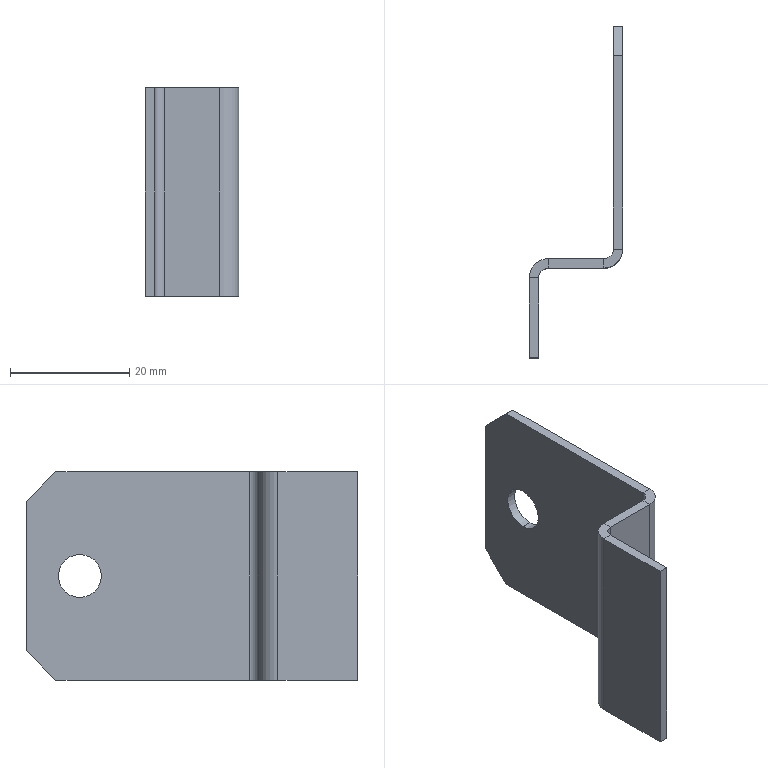Part | SolidWorks | features Chamfer 2, FlatPattern 1, ICE 1, SMBaseFlange 1, SheetMetal 1 | 1 solid | 26 faces | box 15.7 x 55.6 x 35 mm | volume 3683 mm3 | plane 20 | cylinder 6 | commonest cylinder face diameters 3.2 x2 6.4 x2 7.2 x2
STEP:
#1=CARTESIAN_POINT('',(-1.6,47.021,-13.9));
#2=VERTEX_POINT('',#1);
#3=CARTESIAN_POINT('',(-1.6,47.021,-21.1));
#4=VERTEX_POINT('',#3);
#5=CARTESIAN_POINT('',(-1.6,47.021,-17.5));
#6=DIRECTION('',(1.,0.,0.));
#7=DIRECTION('',(0.,0.,-1.));
#8=AXIS2_PLACEMENT_3D('',#5,#6,#7);
#9=CIRCLE('',#8,3.6);
#10=EDGE_CURVE('',#2,#4,#9,.T.);
#11=ORIENTED_EDGE('',*,*,#10,.F.);
#12=CARTESIAN_POINT('',(0.,47.021,-13.9));
#13=VERTEX_POINT('',#12);
#14=CARTESIAN_POINT('',(-1.6,47.021,-13.9));
#15=DIRECTION('',(1.,0.,0.));
#16=VECTOR('',#15,1000.);
#17=LINE('',#14,#16);
#18=EDGE_CURVE('',#2,#13,#17,.T.);
#19=ORIENTED_EDGE('',*,*,#18,.T.);
#20=CARTESIAN_POINT('',(0.,47.021,-21.1));
#21=VERTEX_POINT('',#20);
#22=CARTESIAN_POINT('',(0.,47.021,-17.5));
#23=DIRECTION('',(1.,0.,0.));
#24=DIRECTION('',(0.,0.,-1.));
#25=AXIS2_PLACEMENT_3D('',#22,#23,#24);
#26=CIRCLE('',#25,3.6);
#27=EDGE_CURVE('',#13,#21,#26,.T.);
#28=ORIENTED_EDGE('',*,*,#27,.T.);
#29=CARTESIAN_POINT('',(-1.6,47.021,-21.1));
#30=DIRECTION('',(1.,0.,0.));
#31=VECTOR('',#30,1000.);
#32=LINE('',#29,#31);
#33=EDGE_CURVE('',#4,#21,#32,.T.);
#34=ORIENTED_EDGE('',*,*,#33,.F.);
#35=EDGE_LOOP('',(#11,#19,#28,#34));
#36=FACE_OUTER_BOUND('',#35,.T.);
#37=CARTESIAN_POINT('',(-1.6,47.021,-17.5));
#38=DIRECTION('',(1.,0.,0.));
#39=DIRECTION('',(0.,0.,-1.));
#40=AXIS2_PLACEMENT_3D('',#37,#38,#39);
#41=CYLINDRICAL_SURFACE('',#40,3.6);
#42=ADVANCED_FACE('',(#36),#41,.F.);
#43=CARTESIAN_POINT('',(0.,18.621,-35.));
#44=VERTEX_POINT('',#43);
#45=CARTESIAN_POINT('',(-1.6,18.621,-35.));
#46=VERTEX_POINT('',#45);
#47=CARTESIAN_POINT('',(0.,18.621,-35.));
#48=DIRECTION('',(-1.,0.,0.));
#49=VECTOR('',#48,1000.);
#50=LINE('',#47,#49);
#51=EDGE_CURVE('',#44,#46,#50,.T.);
#52=ORIENTED_EDGE('',*,*,#51,.F.);
#53=CARTESIAN_POINT('',(-3.2,15.421,-35.));
#54=VERTEX_POINT('',#53);
#55=CARTESIAN_POINT('',(-3.2,18.621,-35.));
#56=DIRECTION('',(0.,0.,-1.));
#57=DIRECTION('',(1.,0.,0.));
#58=AXIS2_PLACEMENT_3D('',#55,#56,#57);
#59=CIRCLE('',#58,3.2);
#60=EDGE_CURVE('',#44,#54,#59,.T.);
#61=ORIENTED_EDGE('',*,*,#60,.T.);
#62=CARTESIAN_POINT('',(-3.2,17.021,-35.));
#63=VERTEX_POINT('',#62);
#64=CARTESIAN_POINT('',(-3.2,17.021,-35.));
#65=DIRECTION('',(0.,-1.,0.));
#66=VECTOR('',#65,1000.);
#67=LINE('',#64,#66);
#68=EDGE_CURVE('',#63,#54,#67,.T.);
#69=ORIENTED_EDGE('',*,*,#68,.F.);
#70=CARTESIAN_POINT('',(-3.2,18.621,-35.));
#71=DIRECTION('',(0.,0.,-1.));
#72=DIRECTION('',(1.,0.,0.));
#73=AXIS2_PLACEMENT_3D('',#70,#71,#72);
#74=CIRCLE('',#73,1.6);
#75=EDGE_CURVE('',#46,#63,#74,.T.);
#76=ORIENTED_EDGE('',*,*,#75,.F.);
#77=EDGE_LOOP('',(#52,#61,#69,#76));
#78=FACE_OUTER_BOUND('',#77,.T.);
#79=CARTESIAN_POINT('',(0.,18.621,-35.));
#80=DIRECTION('',(0.,0.,-1.));
#81=DIRECTION('',(-1.,0.,0.));
#82=AXIS2_PLACEMENT_3D('',#79,#80,#81);
#83=PLANE('',#82);
#84=ADVANCED_FACE('',(#78),#83,.T.);
#85=CARTESIAN_POINT('',(-1.6,51.021,-35.));
#86=VERTEX_POINT('',#85);
#87=CARTESIAN_POINT('',(-1.6,56.021,-35.));
#88=DIRECTION('',(0.,-1.,0.));
#89=VECTOR('',#88,1000.);
#90=LINE('',#87,#89);
#91=EDGE_CURVE('',#86,#46,#90,.T.);
#92=ORIENTED_EDGE('',*,*,#91,.F.);
#93=CARTESIAN_POINT('',(0.,51.021,-35.));
#94=VERTEX_POINT('',#93);
#95=CARTESIAN_POINT('',(0.,51.021,-35.));
#96=DIRECTION('',(1.,0.,0.));
#97=VECTOR('',#96,1000.);
#98=LINE('',#95,#97);
#99=EDGE_CURVE('',#86,#94,#98,.T.);
#100=ORIENTED_EDGE('',*,*,#99,.T.);
#101=CARTESIAN_POINT('',(0.,56.021,-35.));
#102=DIRECTION('',(0.,-1.,0.));
#103=VECTOR('',#102,1000.);
#104=LINE('',#101,#103);
#105=EDGE_CURVE('',#94,#44,#104,.T.);
#106=ORIENTED_EDGE('',*,*,#105,.T.);
#107=ORIENTED_EDGE('',*,*,#51,.T.);
#108=EDGE_LOOP('',(#92,#100,#106,#107));
#109=FACE_OUTER_BOUND('',#108,.T.);
#110=CARTESIAN_POINT('',(-3.2,17.021,-35.));
#111=DIRECTION('',(0.,0.,-1.));
#112=DIRECTION('',(-1.,0.,0.));
#113=AXIS2_PLACEMENT_3D('',#110,#111,#112);
#114=PLANE('',#113);
#115=ADVANCED_FACE('',(#109),#114,.T.);
#116=CARTESIAN_POINT('',(-3.2,15.421,0.));
#117=VERTEX_POINT('',#116);
#118=CARTESIAN_POINT('',(-3.2,17.021,0.));
#119=VERTEX_POINT('',#118);
#120=CARTESIAN_POINT('',(-3.2,15.421,0.));
#121=DIRECTION('',(0.,1.,0.));
#122=VECTOR('',#121,1000.);
#123=LINE('',#120,#122);
#124=EDGE_CURVE('',#117,#119,#123,.T.);
#125=ORIENTED_EDGE('',*,*,#124,.F.);
#126=CARTESIAN_POINT('',(0.,18.621,0.));
#127=VERTEX_POINT('',#126);
#128=CARTESIAN_POINT('',(-3.2,18.621,0.));
#129=DIRECTION('',(0.,0.,-1.));
#130=DIRECTION('',(1.,0.,0.));
#131=AXIS2_PLACEMENT_3D('',#128,#129,#130);
#132=CIRCLE('',#131,3.2);
#133=EDGE_CURVE('',#127,#117,#132,.T.);
#134=ORIENTED_EDGE('',*,*,#133,.F.);
#135=CARTESIAN_POINT('',(-1.6,18.621,0.));
#136=VERTEX_POINT('',#135);
#137=CARTESIAN_POINT('',(-1.6,18.621,0.));
#138=DIRECTION('',(1.,0.,0.));
#139=VECTOR('',#138,1000.);
#140=LINE('',#137,#139);
#141=EDGE_CURVE('',#136,#127,#140,.T.);
#142=ORIENTED_EDGE('',*,*,#141,.F.);
#143=CARTESIAN_POINT('',(-3.2,18.621,0.));
#144=DIRECTION('',(0.,0.,-1.));
#145=DIRECTION('',(1.,0.,0.));
#146=AXIS2_PLACEMENT_3D('',#143,#144,#145);
#147=CIRCLE('',#146,1.6);
#148=EDGE_CURVE('',#136,#119,#147,.T.);
#149=ORIENTED_EDGE('',*,*,#148,.T.);
#150=EDGE_LOOP('',(#125,#134,#142,#149));
#151=FACE_OUTER_BOUND('',#150,.T.);
#152=CARTESIAN_POINT('',(-3.2,15.421,0.));
#153=DIRECTION('',(0.,0.,1.));
#154=DIRECTION('',(1.,0.,0.));
#155=AXIS2_PLACEMENT_3D('',#152,#153,#154);
#156=PLANE('',#155);
#157=ADVANCED_FACE('',(#151),#156,.T.);
#158=CARTESIAN_POINT('',(-12.5,15.421,0.));
#159=VERTEX_POINT('',#158);
#160=CARTESIAN_POINT('',(0.,15.421,0.));
#161=DIRECTION('',(-1.,0.,0.));
#162=VECTOR('',#161,1000.);
#163=LINE('',#160,#162);
#164=EDGE_CURVE('',#117,#159,#163,.T.);
#165=ORIENTED_EDGE('',*,*,#164,.F.);
#166=ORIENTED_EDGE('',*,*,#124,.T.);
#167=CARTESIAN_POINT('',(-12.5,17.021,0.));
#168=VERTEX_POINT('',#167);
#169=CARTESIAN_POINT('',(0.,17.021,0.));
#170=DIRECTION('',(-1.,0.,0.));
#171=VECTOR('',#170,1000.);
#172=LINE('',#169,#171);
#173=EDGE_CURVE('',#119,#168,#172,.T.);
#174=ORIENTED_EDGE('',*,*,#173,.T.);
#175=CARTESIAN_POINT('',(-12.5,17.021,0.));
#176=DIRECTION('',(0.,-1.,0.));
#177=VECTOR('',#176,1000.);
#178=LINE('',#175,#177);
#179=EDGE_CURVE('',#168,#159,#178,.T.);
#180=ORIENTED_EDGE('',*,*,#179,.T.);
#181=EDGE_LOOP('',(#165,#166,#174,#180));
#182=FACE_OUTER_BOUND('',#181,.T.);
#183=CARTESIAN_POINT('',(-1.6,18.621,0.));
#184=DIRECTION('',(0.,0.,1.));
#185=DIRECTION('',(1.,0.,0.));
#186=AXIS2_PLACEMENT_3D('',#183,#184,#185);
#187=PLANE('',#186);
#188=ADVANCED_FACE('',(#182),#187,.T.);
#189=CARTESIAN_POINT('',(-12.5,15.421,-35.));
#190=VERTEX_POINT('',#189);
#191=CARTESIAN_POINT('',(-12.5,17.021,-35.));
#192=VERTEX_POINT('',#191);
#193=CARTESIAN_POINT('',(-12.5,15.421,-35.));
#194=DIRECTION('',(0.,1.,0.));
#195=VECTOR('',#194,1000.);
#196=LINE('',#193,#195);
#197=EDGE_CURVE('',#190,#192,#196,.T.);
#198=ORIENTED_EDGE('',*,*,#197,.F.);
#199=CARTESIAN_POINT('',(-14.1,13.821,-35.));
#200=VERTEX_POINT('',#199);
#201=CARTESIAN_POINT('',(-12.5,13.821,-35.));
#202=DIRECTION('',(0.,0.,1.));
#203=DIRECTION('',(-1.,0.,0.));
#204=AXIS2_PLACEMENT_3D('',#201,#202,#203);
#205=CIRCLE('',#204,1.6);
#206=EDGE_CURVE('',#190,#200,#205,.T.);
#207=ORIENTED_EDGE('',*,*,#206,.T.);
#208=CARTESIAN_POINT('',(-15.7,13.821,-35.));
#209=VERTEX_POINT('',#208);
#210=CARTESIAN_POINT('',(-15.7,13.821,-35.));
#211=DIRECTION('',(1.,0.,0.));
#212=VECTOR('',#211,1000.);
#213=LINE('',#210,#212);
#214=EDGE_CURVE('',#209,#200,#213,.T.);
#215=ORIENTED_EDGE('',*,*,#214,.F.);
#216=CARTESIAN_POINT('',(-12.5,13.821,-35.));
#217=DIRECTION('',(0.,0.,1.));
#218=DIRECTION('',(1.,0.,0.));
#219=AXIS2_PLACEMENT_3D('',#216,#217,#218);
#220=CIRCLE('',#219,3.2);
#221=EDGE_CURVE('',#192,#209,#220,.T.);
#222=ORIENTED_EDGE('',*,*,#221,.F.);
#223=EDGE_LOOP('',(#198,#207,#215,#222));
#224=FACE_OUTER_BOUND('',#223,.T.);
#225=CARTESIAN_POINT('',(-12.5,15.421,-35.));
#226=DIRECTION('',(0.,0.,-1.));
#227=DIRECTION('',(-1.,0.,0.));
#228=AXIS2_PLACEMENT_3D('',#225,#226,#227);
#229=PLANE('',#228);
#230=ADVANCED_FACE('',(#224),#229,.T.);
#231=CARTESIAN_POINT('',(0.,15.421,-35.));
#232=DIRECTION('',(-1.,0.,0.));
#233=VECTOR('',#232,1000.);
#234=LINE('',#231,#233);
#235=EDGE_CURVE('',#54,#190,#234,.T.);
#236=ORIENTED_EDGE('',*,*,#235,.T.);
#237=ORIENTED_EDGE('',*,*,#197,.T.);
#238=CARTESIAN_POINT('',(0.,17.021,-35.));
#239=DIRECTION('',(-1.,0.,0.));
#240=VECTOR('',#239,1000.);
#241=LINE('',#238,#240);
#242=EDGE_CURVE('',#63,#192,#241,.T.);
#243=ORIENTED_EDGE('',*,*,#242,.F.);
#244=ORIENTED_EDGE('',*,*,#68,.T.);
#245=EDGE_LOOP('',(#236,#237,#243,#244));
#246=FACE_OUTER_BOUND('',#245,.T.);
#247=CARTESIAN_POINT('',(-15.7,13.821,-35.));
#248=DIRECTION('',(0.,0.,-1.));
#249=DIRECTION('',(-1.,0.,0.));
#250=AXIS2_PLACEMENT_3D('',#247,#248,#249);
#251=PLANE('',#250);
#252=ADVANCED_FACE('',(#246),#251,.T.);
#253=CARTESIAN_POINT('',(-14.1,13.821,0.));
#254=VERTEX_POINT('',#253);
#255=CARTESIAN_POINT('',(-15.7,13.821,0.));
#256=VERTEX_POINT('',#255);
#257=CARTESIAN_POINT('',(-14.1,13.821,0.));
#258=DIRECTION('',(-1.,0.,0.));
#259=VECTOR('',#258,1000.);
#260=LINE('',#257,#259);
#261=EDGE_CURVE('',#254,#256,#260,.T.);
#262=ORIENTED_EDGE('',*,*,#261,.F.);
#263=CARTESIAN_POINT('',(-12.5,13.821,0.));
#264=DIRECTION('',(0.,0.,1.));
#265=DIRECTION('',(-1.,0.,0.));
#266=AXIS2_PLACEMENT_3D('',#263,#264,#265);
#267=CIRCLE('',#266,1.6);
#268=EDGE_CURVE('',#159,#254,#267,.T.);
#269=ORIENTED_EDGE('',*,*,#268,.F.);
#270=ORIENTED_EDGE('',*,*,#179,.F.);
#271=CARTESIAN_POINT('',(-12.5,13.821,0.));
#272=DIRECTION('',(0.,0.,1.));
#273=DIRECTION('',(1.,0.,0.));
#274=AXIS2_PLACEMENT_3D('',#271,#272,#273);
#275=CIRCLE('',#274,3.2);
#276=EDGE_CURVE('',#168,#256,#275,.T.);
#277=ORIENTED_EDGE('',*,*,#276,.T.);
#278=EDGE_LOOP('',(#262,#269,#270,#277));
#279=FACE_OUTER_BOUND('',#278,.T.);
#280=CARTESIAN_POINT('',(-14.1,13.821,0.));
#281=DIRECTION('',(0.,0.,1.));
#282=DIRECTION('',(1.,0.,0.));
#283=AXIS2_PLACEMENT_3D('',#280,#281,#282);
#284=PLANE('',#283);
#285=ADVANCED_FACE('',(#279),#284,.T.);
#286=CARTESIAN_POINT('',(-14.1,0.4211,0.));
#287=VERTEX_POINT('',#286);
#288=CARTESIAN_POINT('',(-14.1,15.421,0.));
#289=DIRECTION('',(0.,-1.,0.));
#290=VECTOR('',#289,1000.);
#291=LINE('',#288,#290);
#292=EDGE_CURVE('',#254,#287,#291,.T.);
#293=ORIENTED_EDGE('',*,*,#292,.F.);
#294=ORIENTED_EDGE('',*,*,#261,.T.);
#295=CARTESIAN_POINT('',(-15.7,0.4211,0.));
#296=VERTEX_POINT('',#295);
#297=CARTESIAN_POINT('',(-15.7,15.421,0.));
#298=DIRECTION('',(0.,-1.,0.));
#299=VECTOR('',#298,1000.);
#300=LINE('',#297,#299);
#301=EDGE_CURVE('',#256,#296,#300,.T.);
#302=ORIENTED_EDGE('',*,*,#301,.T.);
#303=CARTESIAN_POINT('',(-14.1,0.4211,0.));
#304=DIRECTION('',(-1.,0.,0.));
#305=VECTOR('',#304,1000.);
#306=LINE('',#303,#305);
#307=EDGE_CURVE('',#287,#296,#306,.T.);
#308=ORIENTED_EDGE('',*,*,#307,.F.);
#309=EDGE_LOOP('',(#293,#294,#302,#308));
#310=FACE_OUTER_BOUND('',#309,.T.);
#311=CARTESIAN_POINT('',(-12.5,17.021,0.));
#312=DIRECTION('',(0.,0.,1.));
#313=DIRECTION('',(1.,0.,0.));
#314=AXIS2_PLACEMENT_3D('',#311,#312,#313);
#315=PLANE('',#314);
#316=ADVANCED_FACE('',(#310),#315,.T.);
#317=ORIENTED_EDGE('',*,*,#301,.F.);
#318=CARTESIAN_POINT('',(-15.7,13.821,-35.));
#319=DIRECTION('',(0.,0.,1.));
#320=VECTOR('',#319,1000.);
#321=LINE('',#318,#320);
#322=EDGE_CURVE('',#209,#256,#321,.T.);
#323=ORIENTED_EDGE('',*,*,#322,.F.);
#324=CARTESIAN_POINT('',(-15.7,0.4211,-35.));
#325=VERTEX_POINT('',#324);
#326=CARTESIAN_POINT('',(-15.7,15.421,-35.));
#327=DIRECTION('',(0.,-1.,0.));
#328=VECTOR('',#327,1000.);
#329=LINE('',#326,#328);
#330=EDGE_CURVE('',#209,#325,#329,.T.);
#331=ORIENTED_EDGE('',*,*,#330,.T.);
#332=CARTESIAN_POINT('',(-15.7,0.4211,-35.));
#333=DIRECTION('',(0.,0.,1.));
#334=VECTOR('',#333,1000.);
#335=LINE('',#332,#334);
#336=EDGE_CURVE('',#325,#296,#335,.T.);
#337=ORIENTED_EDGE('',*,*,#336,.T.);
#338=EDGE_LOOP('',(#317,#323,#331,#337));
#339=FACE_OUTER_BOUND('',#338,.T.);
#340=CARTESIAN_POINT('',(-15.7,15.421,-35.));
#341=DIRECTION('',(-1.,0.,0.));
#342=DIRECTION('',(0.,0.,1.));
#343=AXIS2_PLACEMENT_3D('',#340,#341,#342);
#344=PLANE('',#343);
#345=ADVANCED_FACE('',(#339),#344,.T.);
#346=ORIENTED_EDGE('',*,*,#276,.F.);
#347=CARTESIAN_POINT('',(-12.5,17.021,-35.));
#348=DIRECTION('',(0.,0.,1.));
#349=VECTOR('',#348,1000.);
#350=LINE('',#347,#349);
#351=EDGE_CURVE('',#192,#168,#350,.T.);
#352=ORIENTED_EDGE('',*,*,#351,.F.);
#353=ORIENTED_EDGE('',*,*,#221,.T.);
#354=ORIENTED_EDGE('',*,*,#322,.T.);
#355=EDGE_LOOP('',(#346,#352,#353,#354));
#356=FACE_OUTER_BOUND('',#355,.T.);
#357=CARTESIAN_POINT('',(-12.5,13.821,-35.));
#358=DIRECTION('',(0.,0.,1.));
#359=DIRECTION('',(1.,0.,0.));
#360=AXIS2_PLACEMENT_3D('',#357,#358,#359);
#361=CYLINDRICAL_SURFACE('',#360,3.2);
#362=ADVANCED_FACE('',(#356),#361,.T.);
#363=ORIENTED_EDGE('',*,*,#173,.F.);
#364=CARTESIAN_POINT('',(-3.2,17.021,-35.));
#365=DIRECTION('',(0.,0.,1.));
#366=VECTOR('',#365,1000.);
#367=LINE('',#364,#366);
#368=EDGE_CURVE('',#63,#119,#367,.T.);
#369=ORIENTED_EDGE('',*,*,#368,.F.);
#370=ORIENTED_EDGE('',*,*,#242,.T.);
#371=ORIENTED_EDGE('',*,*,#351,.T.);
#372=EDGE_LOOP('',(#363,#369,#370,#371));
#373=FACE_OUTER_BOUND('',#372,.T.);
#374=CARTESIAN_POINT('',(0.,17.021,-35.));
#375=DIRECTION('',(0.,1.,0.));
#376=DIRECTION('',(-1.,0.,0.));
#377=AXIS2_PLACEMENT_3D('',#374,#375,#376);
#378=PLANE('',#377);
#379=ADVANCED_FACE('',(#373),#378,.T.);
#380=ORIENTED_EDGE('',*,*,#148,.F.);
#381=CARTESIAN_POINT('',(-1.6,18.621,-35.));
#382=DIRECTION('',(0.,0.,1.));
#383=VECTOR('',#382,1000.);
#384=LINE('',#381,#383);
#385=EDGE_CURVE('',#46,#136,#384,.T.);
#386=ORIENTED_EDGE('',*,*,#385,.F.);
#387=ORIENTED_EDGE('',*,*,#75,.T.);
#388=ORIENTED_EDGE('',*,*,#368,.T.);
#389=EDGE_LOOP('',(#380,#386,#387,#388));
#390=FACE_OUTER_BOUND('',#389,.T.);
#391=CARTESIAN_POINT('',(-3.2,18.621,-35.));
#392=DIRECTION('',(0.,0.,1.));
#393=DIRECTION('',(1.,0.,0.));
#394=AXIS2_PLACEMENT_3D('',#391,#392,#393);
#395=CYLINDRICAL_SURFACE('',#394,1.6);
#396=ADVANCED_FACE('',(#390),#395,.F.);
#397=CARTESIAN_POINT('',(-1.6,47.021,-17.5));
#398=DIRECTION('',(1.,0.,0.));
#399=DIRECTION('',(0.,0.,-1.));
#400=AXIS2_PLACEMENT_3D('',#397,#398,#399);
#401=CIRCLE('',#400,3.6);
#402=EDGE_CURVE('',#4,#2,#401,.T.);
#403=ORIENTED_EDGE('',*,*,#402,.T.);
#404=ORIENTED_EDGE('',*,*,#10,.T.);
#405=EDGE_LOOP('',(#403,#404));
#406=FACE_BOUND('',#405,.T.);
#407=CARTESIAN_POINT('',(-1.6,51.021,0.));
#408=VERTEX_POINT('',#407);
#409=CARTESIAN_POINT('',(-1.6,56.021,0.));
#410=DIRECTION('',(0.,-1.,0.));
#411=VECTOR('',#410,1000.);
#412=LINE('',#409,#411);
#413=EDGE_CURVE('',#408,#136,#412,.T.);
#414=ORIENTED_EDGE('',*,*,#413,.F.);
#415=CARTESIAN_POINT('',(-1.6,56.021,-5.));
#416=VERTEX_POINT('',#415);
#417=CARTESIAN_POINT('',(-1.6,71.021,-20.));
#418=DIRECTION('',(0.,0.7071,-0.7071));
#419=VECTOR('',#418,1000.);
#420=LINE('',#417,#419);
#421=EDGE_CURVE('',#408,#416,#420,.T.);
#422=ORIENTED_EDGE('',*,*,#421,.T.);
#423=CARTESIAN_POINT('',(-1.6,56.021,-30.));
#424=VERTEX_POINT('',#423);
#425=CARTESIAN_POINT('',(-1.6,56.021,-35.));
#426=DIRECTION('',(0.,0.,1.));
#427=VECTOR('',#426,1000.);
#428=LINE('',#425,#427);
#429=EDGE_CURVE('',#424,#416,#428,.T.);
#430=ORIENTED_EDGE('',*,*,#429,.F.);
#431=CARTESIAN_POINT('',(-1.6,53.521,-32.5));
#432=DIRECTION('',(0.,-0.7071,-0.7071));
#433=VECTOR('',#432,1000.);
#434=LINE('',#431,#433);
#435=EDGE_CURVE('',#424,#86,#434,.T.);
#436=ORIENTED_EDGE('',*,*,#435,.T.);
#437=ORIENTED_EDGE('',*,*,#91,.T.);
#438=ORIENTED_EDGE('',*,*,#385,.T.);
#439=EDGE_LOOP('',(#414,#422,#430,#436,#437,#438));
#440=FACE_OUTER_BOUND('',#439,.T.);
#441=CARTESIAN_POINT('',(-1.6,56.021,-35.));
#442=DIRECTION('',(-1.,0.,0.));
#443=DIRECTION('',(0.,-1.,0.));
#444=AXIS2_PLACEMENT_3D('',#441,#442,#443);
#445=PLANE('',#444);
#446=ADVANCED_FACE('',(#406,#440),#445,.T.);
#447=ORIENTED_EDGE('',*,*,#429,.T.);
#448=CARTESIAN_POINT('',(0.,56.021,-5.));
#449=VERTEX_POINT('',#448);
#450=CARTESIAN_POINT('',(-1.6,56.021,-5.));
#451=DIRECTION('',(1.,0.,0.));
#452=VECTOR('',#451,1000.);
#453=LINE('',#450,#452);
#454=EDGE_CURVE('',#416,#449,#453,.T.);
#455=ORIENTED_EDGE('',*,*,#454,.T.);
#456=CARTESIAN_POINT('',(0.,56.021,-30.));
#457=VERTEX_POINT('',#456);
#458=CARTESIAN_POINT('',(0.,56.021,-35.));
#459=DIRECTION('',(0.,0.,1.));
#460=VECTOR('',#459,1000.);
#461=LINE('',#458,#460);
#462=EDGE_CURVE('',#457,#449,#461,.T.);
#463=ORIENTED_EDGE('',*,*,#462,.F.);
#464=CARTESIAN_POINT('',(-1.6,56.021,-30.));
#465=DIRECTION('',(-1.,0.,0.));
#466=VECTOR('',#465,1000.);
#467=LINE('',#464,#466);
#468=EDGE_CURVE('',#457,#424,#467,.T.);
#469=ORIENTED_EDGE('',*,*,#468,.T.);
#470=EDGE_LOOP('',(#447,#455,#463,#469));
#471=FACE_OUTER_BOUND('',#470,.T.);
#472=CARTESIAN_POINT('',(-1.6,56.021,-35.));
#473=DIRECTION('',(0.,-1.,0.));
#474=DIRECTION('',(0.,0.,-1.));
#475=AXIS2_PLACEMENT_3D('',#472,#473,#474);
#476=PLANE('',#475);
#477=ADVANCED_FACE('',(#471),#476,.F.);
#478=CARTESIAN_POINT('',(0.,47.021,-17.5));
#479=DIRECTION('',(1.,0.,0.));
#480=DIRECTION('',(0.,0.,-1.));
#481=AXIS2_PLACEMENT_3D('',#478,#479,#480);
#482=CIRCLE('',#481,3.6);
#483=EDGE_CURVE('',#21,#13,#482,.T.);
#484=ORIENTED_EDGE('',*,*,#483,.F.);
#485=ORIENTED_EDGE('',*,*,#27,.F.);
#486=EDGE_LOOP('',(#484,#485));
#487=FACE_BOUND('',#486,.T.);
#488=ORIENTED_EDGE('',*,*,#462,.T.);
#489=CARTESIAN_POINT('',(0.,51.021,0.));
#490=VERTEX_POINT('',#489);
#491=CARTESIAN_POINT('',(0.,56.021,-5.));
#492=DIRECTION('',(0.,-0.7071,0.7071));
#493=VECTOR('',#492,1000.);
#494=LINE('',#491,#493);
#495=EDGE_CURVE('',#449,#490,#494,.T.);
#496=ORIENTED_EDGE('',*,*,#495,.T.);
#497=CARTESIAN_POINT('',(0.,56.021,0.));
#498=DIRECTION('',(0.,-1.,0.));
#499=VECTOR('',#498,1000.);
#500=LINE('',#497,#499);
#501=EDGE_CURVE('',#490,#127,#500,.T.);
#502=ORIENTED_EDGE('',*,*,#501,.T.);
#503=CARTESIAN_POINT('',(0.,18.621,-35.));
#504=DIRECTION('',(0.,0.,1.));
#505=VECTOR('',#504,1000.);
#506=LINE('',#503,#505);
#507=EDGE_CURVE('',#44,#127,#506,.T.);
#508=ORIENTED_EDGE('',*,*,#507,.F.);
#509=ORIENTED_EDGE('',*,*,#105,.F.);
#510=CARTESIAN_POINT('',(0.,51.021,-35.));
#511=DIRECTION('',(0.,0.7071,0.7071));
#512=VECTOR('',#511,1000.);
#513=LINE('',#510,#512);
#514=EDGE_CURVE('',#94,#457,#513,.T.);
#515=ORIENTED_EDGE('',*,*,#514,.T.);
#516=EDGE_LOOP('',(#488,#496,#502,#508,#509,#515));
#517=FACE_OUTER_BOUND('',#516,.T.);
#518=CARTESIAN_POINT('',(0.,56.021,-35.));
#519=DIRECTION('',(-1.,0.,0.));
#520=DIRECTION('',(0.,-1.,0.));
#521=AXIS2_PLACEMENT_3D('',#518,#519,#520);
#522=PLANE('',#521);
#523=ADVANCED_FACE('',(#487,#517),#522,.F.);
#524=ORIENTED_EDGE('',*,*,#133,.T.);
#525=CARTESIAN_POINT('',(-3.2,15.421,-35.));
#526=DIRECTION('',(0.,0.,1.));
#527=VECTOR('',#526,1000.);
#528=LINE('',#525,#527);
#529=EDGE_CURVE('',#54,#117,#528,.T.);
#530=ORIENTED_EDGE('',*,*,#529,.F.);
#531=ORIENTED_EDGE('',*,*,#60,.F.);
#532=ORIENTED_EDGE('',*,*,#507,.T.);
#533=EDGE_LOOP('',(#524,#530,#531,#532));
#534=FACE_OUTER_BOUND('',#533,.T.);
#535=CARTESIAN_POINT('',(-3.2,18.621,-35.));
#536=DIRECTION('',(0.,0.,1.));
#537=DIRECTION('',(1.,0.,0.));
#538=AXIS2_PLACEMENT_3D('',#535,#536,#537);
#539=CYLINDRICAL_SURFACE('',#538,3.2);
#540=ADVANCED_FACE('',(#534),#539,.T.);
#541=ORIENTED_EDGE('',*,*,#164,.T.);
#542=CARTESIAN_POINT('',(-12.5,15.421,-35.));
#543=DIRECTION('',(0.,0.,1.));
#544=VECTOR('',#543,1000.);
#545=LINE('',#542,#544);
#546=EDGE_CURVE('',#190,#159,#545,.T.);
#547=ORIENTED_EDGE('',*,*,#546,.F.);
#548=ORIENTED_EDGE('',*,*,#235,.F.);
#549=ORIENTED_EDGE('',*,*,#529,.T.);
#550=EDGE_LOOP('',(#541,#547,#548,#549));
#551=FACE_OUTER_BOUND('',#550,.T.);
#552=CARTESIAN_POINT('',(0.,15.421,-35.));
#553=DIRECTION('',(0.,1.,0.));
#554=DIRECTION('',(-1.,0.,0.));
#555=AXIS2_PLACEMENT_3D('',#552,#553,#554);
#556=PLANE('',#555);
#557=ADVANCED_FACE('',(#551),#556,.F.);
#558=ORIENTED_EDGE('',*,*,#268,.T.);
#559=CARTESIAN_POINT('',(-14.1,13.821,-35.));
#560=DIRECTION('',(0.,0.,1.));
#561=VECTOR('',#560,1000.);
#562=LINE('',#559,#561);
#563=EDGE_CURVE('',#200,#254,#562,.T.);
#564=ORIENTED_EDGE('',*,*,#563,.F.);
#565=ORIENTED_EDGE('',*,*,#206,.F.);
#566=ORIENTED_EDGE('',*,*,#546,.T.);
#567=EDGE_LOOP('',(#558,#564,#565,#566));
#568=FACE_OUTER_BOUND('',#567,.T.);
#569=CARTESIAN_POINT('',(-12.5,13.821,-35.));
#570=DIRECTION('',(0.,0.,1.));
#571=DIRECTION('',(1.,0.,0.));
#572=AXIS2_PLACEMENT_3D('',#569,#570,#571);
#573=CYLINDRICAL_SURFACE('',#572,1.6);
#574=ADVANCED_FACE('',(#568),#573,.F.);
#575=ORIENTED_EDGE('',*,*,#292,.T.);
#576=CARTESIAN_POINT('',(-14.1,0.4211,-35.));
#577=VERTEX_POINT('',#576);
#578=CARTESIAN_POINT('',(-14.1,0.4211,-35.));
#579=DIRECTION('',(0.,0.,1.));
#580=VECTOR('',#579,1000.);
#581=LINE('',#578,#580);
#582=EDGE_CURVE('',#577,#287,#581,.T.);
#583=ORIENTED_EDGE('',*,*,#582,.F.);
#584=CARTESIAN_POINT('',(-14.1,15.421,-35.));
#585=DIRECTION('',(0.,-1.,0.));
#586=VECTOR('',#585,1000.);
#587=LINE('',#584,#586);
#588=EDGE_CURVE('',#200,#577,#587,.T.);
#589=ORIENTED_EDGE('',*,*,#588,.F.);
#590=ORIENTED_EDGE('',*,*,#563,.T.);
#591=EDGE_LOOP('',(#575,#583,#589,#590));
#592=FACE_OUTER_BOUND('',#591,.T.);
#593=CARTESIAN_POINT('',(-14.1,15.421,-35.));
#594=DIRECTION('',(-1.,0.,0.));
#595=DIRECTION('',(0.,0.,1.));
#596=AXIS2_PLACEMENT_3D('',#593,#594,#595);
#597=PLANE('',#596);
#598=ADVANCED_FACE('',(#592),#597,.F.);
#599=ORIENTED_EDGE('',*,*,#307,.T.);
#600=ORIENTED_EDGE('',*,*,#336,.F.);
#601=CARTESIAN_POINT('',(-14.1,0.4211,-35.));
#602=DIRECTION('',(-1.,0.,0.));
#603=VECTOR('',#602,1000.);
#604=LINE('',#601,#603);
#605=EDGE_CURVE('',#577,#325,#604,.T.);
#606=ORIENTED_EDGE('',*,*,#605,.F.);
#607=ORIENTED_EDGE('',*,*,#582,.T.);
#608=EDGE_LOOP('',(#599,#600,#606,#607));
#609=FACE_OUTER_BOUND('',#608,.T.);
#610=CARTESIAN_POINT('',(-14.1,0.4211,-35.));
#611=DIRECTION('',(0.,1.,0.));
#612=DIRECTION('',(0.,0.,1.));
#613=AXIS2_PLACEMENT_3D('',#610,#611,#612);
#614=PLANE('',#613);
#615=ADVANCED_FACE('',(#609),#614,.F.);
#616=ORIENTED_EDGE('',*,*,#330,.F.);
#617=ORIENTED_EDGE('',*,*,#214,.T.);
#618=ORIENTED_EDGE('',*,*,#588,.T.);
#619=ORIENTED_EDGE('',*,*,#605,.T.);
#620=EDGE_LOOP('',(#616,#617,#618,#619));
#621=FACE_OUTER_BOUND('',#620,.T.);
#622=CARTESIAN_POINT('',(-12.5,13.821,-35.));
#623=DIRECTION('',(0.,0.,-1.));
#624=DIRECTION('',(-1.,0.,0.));
#625=AXIS2_PLACEMENT_3D('',#622,#623,#624);
#626=PLANE('',#625);
#627=ADVANCED_FACE('',(#621),#626,.T.);
#628=ORIENTED_EDGE('',*,*,#501,.F.);
#629=CARTESIAN_POINT('',(-12.5,51.021,0.));
#630=DIRECTION('',(-1.,0.,0.));
#631=VECTOR('',#630,1000.);
#632=LINE('',#629,#631);
#633=EDGE_CURVE('',#490,#408,#632,.T.);
#634=ORIENTED_EDGE('',*,*,#633,.T.);
#635=ORIENTED_EDGE('',*,*,#413,.T.);
#636=ORIENTED_EDGE('',*,*,#141,.T.);
#637=EDGE_LOOP('',(#628,#634,#635,#636));
#638=FACE_OUTER_BOUND('',#637,.T.);
#639=CARTESIAN_POINT('',(-12.5,13.821,0.));
#640=DIRECTION('',(0.,0.,-1.));
#641=DIRECTION('',(-1.,0.,0.));
#642=AXIS2_PLACEMENT_3D('',#639,#640,#641);
#643=PLANE('',#642);
#644=ADVANCED_FACE('',(#638),#643,.F.);
#645=ORIENTED_EDGE('',*,*,#435,.F.);
#646=ORIENTED_EDGE('',*,*,#468,.F.);
#647=ORIENTED_EDGE('',*,*,#514,.F.);
#648=ORIENTED_EDGE('',*,*,#99,.F.);
#649=EDGE_LOOP('',(#645,#646,#647,#648));
#650=FACE_OUTER_BOUND('',#649,.T.);
#651=CARTESIAN_POINT('',(-3.2,51.021,-35.));
#652=DIRECTION('',(0.,0.7071,-0.7071));
#653=DIRECTION('',(-1.,0.,0.));
#654=AXIS2_PLACEMENT_3D('',#651,#652,#653);
#655=PLANE('',#654);
#656=ADVANCED_FACE('',(#650),#655,.T.);
#657=ORIENTED_EDGE('',*,*,#421,.F.);
#658=ORIENTED_EDGE('',*,*,#633,.F.);
#659=ORIENTED_EDGE('',*,*,#495,.F.);
#660=ORIENTED_EDGE('',*,*,#454,.F.);
#661=EDGE_LOOP('',(#657,#658,#659,#660));
#662=FACE_OUTER_BOUND('',#661,.T.);
#663=CARTESIAN_POINT('',(-1.6,56.021,-5.));
#664=DIRECTION('',(0.,-0.7071,-0.7071));
#665=DIRECTION('',(1.,0.,0.));
#666=AXIS2_PLACEMENT_3D('',#663,#664,#665);
#667=PLANE('',#666);
#668=ADVANCED_FACE('',(#662),#667,.F.);
#669=ORIENTED_EDGE('',*,*,#18,.F.);
#670=ORIENTED_EDGE('',*,*,#402,.F.);
#671=ORIENTED_EDGE('',*,*,#33,.T.);
#672=ORIENTED_EDGE('',*,*,#483,.T.);
#673=EDGE_LOOP('',(#669,#670,#671,#672));
#674=FACE_OUTER_BOUND('',#673,.T.);
#675=CARTESIAN_POINT('',(-1.6,47.021,-17.5));
#676=DIRECTION('',(1.,0.,0.));
#677=DIRECTION('',(0.,0.,-1.));
#678=AXIS2_PLACEMENT_3D('',#675,#676,#677);
#679=CYLINDRICAL_SURFACE('',#678,3.6);
#680=ADVANCED_FACE('',(#674),#679,.F.);
#681=CLOSED_SHELL('',(#42,#84,#115,#157,#188,#230,#252,#285,#316,#345,#362,#379,#396,#446,#477,#523,#540,#557,#574,#598,#615,#627,#644,#656,#668,#680));
#682=MANIFOLD_SOLID_BREP('',#681);
#683=CARTESIAN_POINT('',(0.,0.,0.));
#684=DIRECTION('',(0.,0.,1.));
#685=DIRECTION('',(1.,0.,0.));
#686=AXIS2_PLACEMENT_3D('',#683,#684,#685);
#687=(LENGTH_UNIT()NAMED_UNIT(*)SI_UNIT(.MILLI.,.METRE.));
#688=UNCERTAINTY_MEASURE_WITH_UNIT(LENGTH_MEASURE(0.00001),#687,'','');
#689=(NAMED_UNIT(*)PLANE_ANGLE_UNIT()SI_UNIT($,.RADIAN.));
#690=(NAMED_UNIT(*)SI_UNIT($,.STERADIAN.)SOLID_ANGLE_UNIT());
#691=(GEOMETRIC_REPRESENTATION_CONTEXT(3)GLOBAL_UNCERTAINTY_ASSIGNED_CONTEXT((#688))GLOBAL_UNIT_ASSIGNED_CONTEXT((#687,#689,#690))REPRESENTATION_CONTEXT('',''));
#692=ADVANCED_BREP_SHAPE_REPRESENTATION('',(#682,#686),#691);